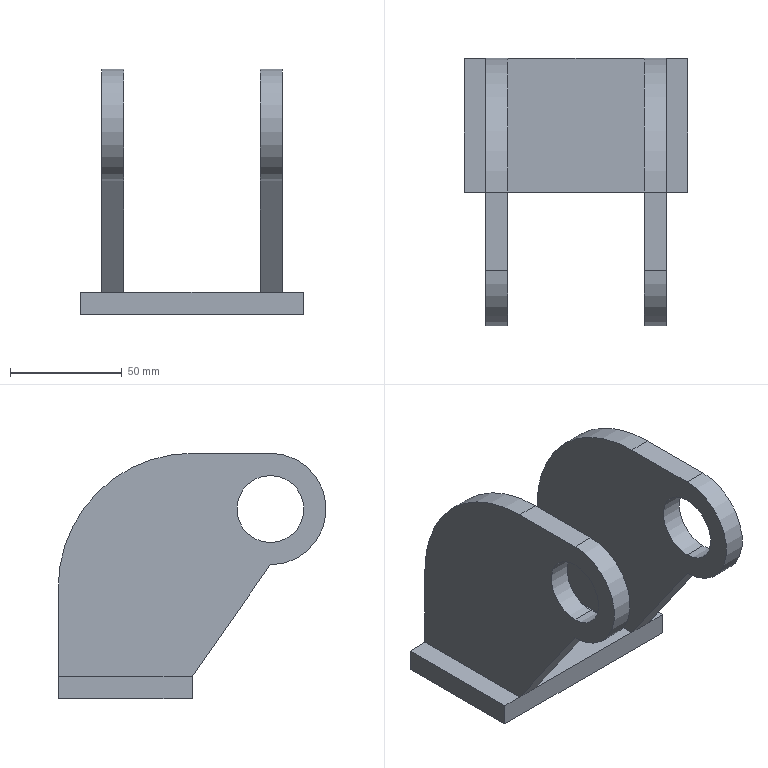Part | STEP file | TN-NHGJQJ-001-002 | 1 solid | 24 faces | box 100 x 120 x 110 mm | volume 222546 mm3 | plane 16 | cylinder 8 | commonest cylinder face diameters 30 x4 50 x2 120 x2
STEP:
#1=CARTESIAN_POINT('',(16.652,-66.545,70.));
#2=VERTEX_POINT('',#1);
#3=CARTESIAN_POINT('',(16.652,-66.545,100.));
#4=VERTEX_POINT('',#3);
#5=CARTESIAN_POINT('',(16.652,-66.545,85.));
#6=DIRECTION('',(-1.,0.,0.));
#7=DIRECTION('',(0.,0.,1.));
#8=AXIS2_PLACEMENT_3D('',#5,#6,#7);
#9=CIRCLE('',#8,15.);
#10=EDGE_CURVE('',#2,#4,#9,.T.);
#11=ORIENTED_EDGE('',*,*,#10,.F.);
#12=CARTESIAN_POINT('',(6.652,-66.545,70.));
#13=VERTEX_POINT('',#12);
#14=CARTESIAN_POINT('',(26.152,-66.545,70.));
#15=DIRECTION('',(-1.,0.,0.));
#16=VECTOR('',#15,1000.);
#17=LINE('',#14,#16);
#18=EDGE_CURVE('',#2,#13,#17,.T.);
#19=ORIENTED_EDGE('',*,*,#18,.T.);
#20=CARTESIAN_POINT('',(6.652,-66.545,100.));
#21=VERTEX_POINT('',#20);
#22=CARTESIAN_POINT('',(6.652,-66.545,85.));
#23=DIRECTION('',(-1.,0.,0.));
#24=DIRECTION('',(0.,0.,1.));
#25=AXIS2_PLACEMENT_3D('',#22,#23,#24);
#26=CIRCLE('',#25,15.);
#27=EDGE_CURVE('',#13,#21,#26,.T.);
#28=ORIENTED_EDGE('',*,*,#27,.T.);
#29=CARTESIAN_POINT('',(26.152,-66.545,100.));
#30=DIRECTION('',(-1.,0.,0.));
#31=VECTOR('',#30,1000.);
#32=LINE('',#29,#31);
#33=EDGE_CURVE('',#4,#21,#32,.T.);
#34=ORIENTED_EDGE('',*,*,#33,.F.);
#35=EDGE_LOOP('',(#11,#19,#28,#34));
#36=FACE_OUTER_BOUND('',#35,.T.);
#37=CARTESIAN_POINT('',(26.152,-66.545,85.));
#38=DIRECTION('',(-1.,0.,0.));
#39=DIRECTION('',(0.,0.,1.));
#40=AXIS2_PLACEMENT_3D('',#37,#38,#39);
#41=CYLINDRICAL_SURFACE('',#40,15.);
#42=ADVANCED_FACE('',(#36),#41,.F.);
#43=CARTESIAN_POINT('',(-54.348,-66.545,100.));
#44=VERTEX_POINT('',#43);
#45=CARTESIAN_POINT('',(-54.348,-66.545,70.));
#46=VERTEX_POINT('',#45);
#47=CARTESIAN_POINT('',(-54.348,-66.545,85.));
#48=DIRECTION('',(1.,0.,0.));
#49=DIRECTION('',(0.,0.,1.));
#50=AXIS2_PLACEMENT_3D('',#47,#48,#49);
#51=CIRCLE('',#50,15.);
#52=EDGE_CURVE('',#44,#46,#51,.T.);
#53=ORIENTED_EDGE('',*,*,#52,.T.);
#54=CARTESIAN_POINT('',(-64.348,-66.545,70.));
#55=VERTEX_POINT('',#54);
#56=CARTESIAN_POINT('',(26.152,-66.545,70.));
#57=DIRECTION('',(-1.,0.,0.));
#58=VECTOR('',#57,1000.);
#59=LINE('',#56,#58);
#60=EDGE_CURVE('',#46,#55,#59,.T.);
#61=ORIENTED_EDGE('',*,*,#60,.T.);
#62=CARTESIAN_POINT('',(-64.348,-66.545,100.));
#63=VERTEX_POINT('',#62);
#64=CARTESIAN_POINT('',(-64.348,-66.545,85.));
#65=DIRECTION('',(-1.,0.,0.));
#66=DIRECTION('',(0.,0.,1.));
#67=AXIS2_PLACEMENT_3D('',#64,#65,#66);
#68=CIRCLE('',#67,15.);
#69=EDGE_CURVE('',#55,#63,#68,.T.);
#70=ORIENTED_EDGE('',*,*,#69,.T.);
#71=CARTESIAN_POINT('',(26.152,-66.545,100.));
#72=DIRECTION('',(-1.,0.,0.));
#73=VECTOR('',#72,1000.);
#74=LINE('',#71,#73);
#75=EDGE_CURVE('',#44,#63,#74,.T.);
#76=ORIENTED_EDGE('',*,*,#75,.F.);
#77=EDGE_LOOP('',(#53,#61,#70,#76));
#78=FACE_OUTER_BOUND('',#77,.T.);
#79=CARTESIAN_POINT('',(26.152,-66.545,85.));
#80=DIRECTION('',(-1.,0.,0.));
#81=DIRECTION('',(0.,0.,1.));
#82=AXIS2_PLACEMENT_3D('',#79,#80,#81);
#83=CYLINDRICAL_SURFACE('',#82,15.);
#84=ADVANCED_FACE('',(#78),#83,.F.);
#85=CARTESIAN_POINT('',(6.652,-66.545,85.));
#86=DIRECTION('',(-1.,0.,0.));
#87=DIRECTION('',(0.,0.,1.));
#88=AXIS2_PLACEMENT_3D('',#85,#86,#87);
#89=CIRCLE('',#88,15.);
#90=EDGE_CURVE('',#21,#13,#89,.T.);
#91=ORIENTED_EDGE('',*,*,#90,.F.);
#92=ORIENTED_EDGE('',*,*,#27,.F.);
#93=EDGE_LOOP('',(#91,#92));
#94=FACE_BOUND('',#93,.T.);
#95=CARTESIAN_POINT('',(6.652,-66.545,60.));
#96=VERTEX_POINT('',#95);
#97=CARTESIAN_POINT('',(6.652,-31.545,10.));
#98=VERTEX_POINT('',#97);
#99=CARTESIAN_POINT('',(6.652,-66.545,60.));
#100=DIRECTION('',(0.,0.5735,-0.8192));
#101=VECTOR('',#100,1000.);
#102=LINE('',#99,#101);
#103=EDGE_CURVE('',#96,#98,#102,.T.);
#104=ORIENTED_EDGE('',*,*,#103,.F.);
#105=CARTESIAN_POINT('',(6.652,-66.545,110.));
#106=VERTEX_POINT('',#105);
#107=CARTESIAN_POINT('',(6.652,-66.545,85.));
#108=DIRECTION('',(1.,0.,0.));
#109=DIRECTION('',(0.,0.,-1.));
#110=AXIS2_PLACEMENT_3D('',#107,#108,#109);
#111=CIRCLE('',#110,25.);
#112=EDGE_CURVE('',#106,#96,#111,.T.);
#113=ORIENTED_EDGE('',*,*,#112,.F.);
#114=CARTESIAN_POINT('',(6.652,-31.545,110.));
#115=VERTEX_POINT('',#114);
#116=CARTESIAN_POINT('',(6.652,28.455,110.));
#117=DIRECTION('',(0.,-1.,0.));
#118=VECTOR('',#117,1000.);
#119=LINE('',#116,#118);
#120=EDGE_CURVE('',#115,#106,#119,.T.);
#121=ORIENTED_EDGE('',*,*,#120,.F.);
#122=CARTESIAN_POINT('',(6.652,28.455,50.));
#123=VERTEX_POINT('',#122);
#124=CARTESIAN_POINT('',(6.652,-31.545,50.));
#125=DIRECTION('',(1.,0.,0.));
#126=DIRECTION('',(0.,0.,-1.));
#127=AXIS2_PLACEMENT_3D('',#124,#125,#126);
#128=CIRCLE('',#127,60.);
#129=EDGE_CURVE('',#123,#115,#128,.T.);
#130=ORIENTED_EDGE('',*,*,#129,.F.);
#131=CARTESIAN_POINT('',(6.652,28.455,10.));
#132=VERTEX_POINT('',#131);
#133=CARTESIAN_POINT('',(6.652,28.455,110.));
#134=DIRECTION('',(0.,0.,1.));
#135=VECTOR('',#134,1000.);
#136=LINE('',#133,#135);
#137=EDGE_CURVE('',#132,#123,#136,.T.);
#138=ORIENTED_EDGE('',*,*,#137,.F.);
#139=CARTESIAN_POINT('',(6.652,28.455,10.));
#140=DIRECTION('',(0.,1.,0.));
#141=VECTOR('',#140,1000.);
#142=LINE('',#139,#141);
#143=EDGE_CURVE('',#98,#132,#142,.T.);
#144=ORIENTED_EDGE('',*,*,#143,.F.);
#145=EDGE_LOOP('',(#104,#113,#121,#130,#138,#144));
#146=FACE_OUTER_BOUND('',#145,.T.);
#147=CARTESIAN_POINT('',(6.652,28.455,110.));
#148=DIRECTION('',(1.,0.,0.));
#149=DIRECTION('',(0.,1.,0.));
#150=AXIS2_PLACEMENT_3D('',#147,#148,#149);
#151=PLANE('',#150);
#152=ADVANCED_FACE('',(#94,#146),#151,.F.);
#153=ORIENTED_EDGE('',*,*,#18,.F.);
#154=CARTESIAN_POINT('',(16.652,-66.545,85.));
#155=DIRECTION('',(-1.,0.,0.));
#156=DIRECTION('',(0.,0.,1.));
#157=AXIS2_PLACEMENT_3D('',#154,#155,#156);
#158=CIRCLE('',#157,15.);
#159=EDGE_CURVE('',#4,#2,#158,.T.);
#160=ORIENTED_EDGE('',*,*,#159,.F.);
#161=ORIENTED_EDGE('',*,*,#33,.T.);
#162=ORIENTED_EDGE('',*,*,#90,.T.);
#163=EDGE_LOOP('',(#153,#160,#161,#162));
#164=FACE_OUTER_BOUND('',#163,.T.);
#165=CARTESIAN_POINT('',(26.152,-66.545,85.));
#166=DIRECTION('',(-1.,0.,0.));
#167=DIRECTION('',(0.,0.,1.));
#168=AXIS2_PLACEMENT_3D('',#165,#166,#167);
#169=CYLINDRICAL_SURFACE('',#168,15.);
#170=ADVANCED_FACE('',(#164),#169,.F.);
#171=CARTESIAN_POINT('',(-54.348,28.455,10.));
#172=VERTEX_POINT('',#171);
#173=CARTESIAN_POINT('',(0.,28.455,10.));
#174=DIRECTION('',(-1.,0.,0.));
#175=VECTOR('',#174,1000.);
#176=LINE('',#173,#175);
#177=EDGE_CURVE('',#132,#172,#176,.T.);
#178=ORIENTED_EDGE('',*,*,#177,.T.);
#179=CARTESIAN_POINT('',(-54.348,-31.545,10.));
#180=VERTEX_POINT('',#179);
#181=CARTESIAN_POINT('',(-54.348,0.,10.));
#182=DIRECTION('',(0.,-1.,0.));
#183=VECTOR('',#182,1000.);
#184=LINE('',#181,#183);
#185=EDGE_CURVE('',#172,#180,#184,.T.);
#186=ORIENTED_EDGE('',*,*,#185,.T.);
#187=CARTESIAN_POINT('',(0.,-31.545,10.));
#188=DIRECTION('',(1.,0.,0.));
#189=VECTOR('',#188,1000.);
#190=LINE('',#187,#189);
#191=EDGE_CURVE('',#180,#98,#190,.T.);
#192=ORIENTED_EDGE('',*,*,#191,.T.);
#193=ORIENTED_EDGE('',*,*,#143,.T.);
#194=EDGE_LOOP('',(#178,#186,#192,#193));
#195=FACE_OUTER_BOUND('',#194,.T.);
#196=CARTESIAN_POINT('',(0.,0.,10.));
#197=DIRECTION('',(0.,0.,1.));
#198=DIRECTION('',(1.,0.,0.));
#199=AXIS2_PLACEMENT_3D('',#196,#197,#198);
#200=PLANE('',#199);
#201=ADVANCED_FACE('',(#195),#200,.T.);
#202=ORIENTED_EDGE('',*,*,#103,.T.);
#203=CARTESIAN_POINT('',(16.652,-31.545,10.));
#204=VERTEX_POINT('',#203);
#205=CARTESIAN_POINT('',(6.652,-31.545,10.));
#206=DIRECTION('',(1.,0.,0.));
#207=VECTOR('',#206,1000.);
#208=LINE('',#205,#207);
#209=EDGE_CURVE('',#98,#204,#208,.T.);
#210=ORIENTED_EDGE('',*,*,#209,.T.);
#211=CARTESIAN_POINT('',(16.652,-66.545,60.));
#212=VERTEX_POINT('',#211);
#213=CARTESIAN_POINT('',(16.652,-31.545,10.));
#214=DIRECTION('',(0.,-0.5735,0.8192));
#215=VECTOR('',#214,1000.);
#216=LINE('',#213,#215);
#217=EDGE_CURVE('',#204,#212,#216,.T.);
#218=ORIENTED_EDGE('',*,*,#217,.T.);
#219=CARTESIAN_POINT('',(6.652,-66.545,60.));
#220=DIRECTION('',(-1.,0.,0.));
#221=VECTOR('',#220,1000.);
#222=LINE('',#219,#221);
#223=EDGE_CURVE('',#212,#96,#222,.T.);
#224=ORIENTED_EDGE('',*,*,#223,.T.);
#225=EDGE_LOOP('',(#202,#210,#218,#224));
#226=FACE_OUTER_BOUND('',#225,.T.);
#227=CARTESIAN_POINT('',(6.652,-31.545,10.));
#228=DIRECTION('',(0.,-0.8192,-0.5735));
#229=DIRECTION('',(0.,0.5735,-0.8192));
#230=AXIS2_PLACEMENT_3D('',#227,#228,#229);
#231=PLANE('',#230);
#232=ADVANCED_FACE('',(#226),#231,.T.);
#233=CARTESIAN_POINT('',(16.652,-66.545,110.));
#234=VERTEX_POINT('',#233);
#235=CARTESIAN_POINT('',(16.652,-66.545,85.));
#236=DIRECTION('',(-1.,0.,0.));
#237=DIRECTION('',(0.,0.,-1.));
#238=AXIS2_PLACEMENT_3D('',#235,#236,#237);
#239=CIRCLE('',#238,25.);
#240=EDGE_CURVE('',#212,#234,#239,.T.);
#241=ORIENTED_EDGE('',*,*,#240,.T.);
#242=CARTESIAN_POINT('',(0.,-66.545,110.));
#243=DIRECTION('',(-1.,0.,0.));
#244=VECTOR('',#243,1000.);
#245=LINE('',#242,#244);
#246=EDGE_CURVE('',#234,#106,#245,.T.);
#247=ORIENTED_EDGE('',*,*,#246,.T.);
#248=ORIENTED_EDGE('',*,*,#112,.T.);
#249=ORIENTED_EDGE('',*,*,#223,.F.);
#250=EDGE_LOOP('',(#241,#247,#248,#249));
#251=FACE_OUTER_BOUND('',#250,.T.);
#252=CARTESIAN_POINT('',(0.,-66.545,85.));
#253=DIRECTION('',(1.,0.,0.));
#254=DIRECTION('',(0.,0.,-1.));
#255=AXIS2_PLACEMENT_3D('',#252,#253,#254);
#256=CYLINDRICAL_SURFACE('',#255,25.);
#257=ADVANCED_FACE('',(#251),#256,.T.);
#258=CARTESIAN_POINT('',(16.652,-31.545,110.));
#259=VERTEX_POINT('',#258);
#260=CARTESIAN_POINT('',(16.652,0.,110.));
#261=DIRECTION('',(0.,1.,0.));
#262=VECTOR('',#261,1000.);
#263=LINE('',#260,#262);
#264=EDGE_CURVE('',#234,#259,#263,.T.);
#265=ORIENTED_EDGE('',*,*,#264,.T.);
#266=CARTESIAN_POINT('',(0.,-31.545,110.));
#267=DIRECTION('',(-1.,0.,0.));
#268=VECTOR('',#267,1000.);
#269=LINE('',#266,#268);
#270=EDGE_CURVE('',#259,#115,#269,.T.);
#271=ORIENTED_EDGE('',*,*,#270,.T.);
#272=ORIENTED_EDGE('',*,*,#120,.T.);
#273=ORIENTED_EDGE('',*,*,#246,.F.);
#274=EDGE_LOOP('',(#265,#271,#272,#273));
#275=FACE_OUTER_BOUND('',#274,.T.);
#276=CARTESIAN_POINT('',(0.,0.,110.));
#277=DIRECTION('',(0.,0.,1.));
#278=DIRECTION('',(1.,0.,0.));
#279=AXIS2_PLACEMENT_3D('',#276,#277,#278);
#280=PLANE('',#279);
#281=ADVANCED_FACE('',(#275),#280,.T.);
#282=ORIENTED_EDGE('',*,*,#129,.T.);
#283=ORIENTED_EDGE('',*,*,#270,.F.);
#284=CARTESIAN_POINT('',(16.652,28.455,50.));
#285=VERTEX_POINT('',#284);
#286=CARTESIAN_POINT('',(16.652,-31.545,50.));
#287=DIRECTION('',(-1.,0.,0.));
#288=DIRECTION('',(0.,0.,-1.));
#289=AXIS2_PLACEMENT_3D('',#286,#287,#288);
#290=CIRCLE('',#289,60.);
#291=EDGE_CURVE('',#259,#285,#290,.T.);
#292=ORIENTED_EDGE('',*,*,#291,.T.);
#293=CARTESIAN_POINT('',(0.,28.455,50.));
#294=DIRECTION('',(-1.,0.,0.));
#295=VECTOR('',#294,1000.);
#296=LINE('',#293,#295);
#297=EDGE_CURVE('',#285,#123,#296,.T.);
#298=ORIENTED_EDGE('',*,*,#297,.T.);
#299=EDGE_LOOP('',(#282,#283,#292,#298));
#300=FACE_OUTER_BOUND('',#299,.T.);
#301=CARTESIAN_POINT('',(0.,-31.545,50.));
#302=DIRECTION('',(1.,0.,0.));
#303=DIRECTION('',(0.,0.,-1.));
#304=AXIS2_PLACEMENT_3D('',#301,#302,#303);
#305=CYLINDRICAL_SURFACE('',#304,60.);
#306=ADVANCED_FACE('',(#300),#305,.T.);
#307=ORIENTED_EDGE('',*,*,#297,.F.);
#308=CARTESIAN_POINT('',(16.652,28.455,10.));
#309=VERTEX_POINT('',#308);
#310=CARTESIAN_POINT('',(16.652,28.455,10.));
#311=DIRECTION('',(0.,0.,1.));
#312=VECTOR('',#311,1000.);
#313=LINE('',#310,#312);
#314=EDGE_CURVE('',#309,#285,#313,.T.);
#315=ORIENTED_EDGE('',*,*,#314,.F.);
#316=CARTESIAN_POINT('',(26.152,28.455,10.));
#317=VERTEX_POINT('',#316);
#318=CARTESIAN_POINT('',(-73.848,28.455,10.));
#319=DIRECTION('',(-1.,0.,0.));
#320=VECTOR('',#319,1000.);
#321=LINE('',#318,#320);
#322=EDGE_CURVE('',#317,#309,#321,.T.);
#323=ORIENTED_EDGE('',*,*,#322,.F.);
#324=CARTESIAN_POINT('',(26.152,28.455,0.));
#325=VERTEX_POINT('',#324);
#326=CARTESIAN_POINT('',(26.152,28.455,10.));
#327=DIRECTION('',(0.,0.,1.));
#328=VECTOR('',#327,1000.);
#329=LINE('',#326,#328);
#330=EDGE_CURVE('',#325,#317,#329,.T.);
#331=ORIENTED_EDGE('',*,*,#330,.F.);
#332=CARTESIAN_POINT('',(-73.848,28.455,0.));
#333=VERTEX_POINT('',#332);
#334=CARTESIAN_POINT('',(-73.848,28.455,0.));
#335=DIRECTION('',(1.,0.,0.));
#336=VECTOR('',#335,1000.);
#337=LINE('',#334,#336);
#338=EDGE_CURVE('',#333,#325,#337,.T.);
#339=ORIENTED_EDGE('',*,*,#338,.F.);
#340=CARTESIAN_POINT('',(-73.848,28.455,10.));
#341=VERTEX_POINT('',#340);
#342=CARTESIAN_POINT('',(-73.848,28.455,10.));
#343=DIRECTION('',(0.,0.,-1.));
#344=VECTOR('',#343,1000.);
#345=LINE('',#342,#344);
#346=EDGE_CURVE('',#341,#333,#345,.T.);
#347=ORIENTED_EDGE('',*,*,#346,.F.);
#348=CARTESIAN_POINT('',(-64.348,28.455,10.));
#349=VERTEX_POINT('',#348);
#350=CARTESIAN_POINT('',(-73.848,28.455,10.));
#351=DIRECTION('',(-1.,0.,0.));
#352=VECTOR('',#351,1000.);
#353=LINE('',#350,#352);
#354=EDGE_CURVE('',#349,#341,#353,.T.);
#355=ORIENTED_EDGE('',*,*,#354,.F.);
#356=CARTESIAN_POINT('',(-64.348,28.455,50.));
#357=VERTEX_POINT('',#356);
#358=CARTESIAN_POINT('',(-64.348,28.455,10.));
#359=DIRECTION('',(0.,0.,-1.));
#360=VECTOR('',#359,1000.);
#361=LINE('',#358,#360);
#362=EDGE_CURVE('',#357,#349,#361,.T.);
#363=ORIENTED_EDGE('',*,*,#362,.F.);
#364=CARTESIAN_POINT('',(-54.348,28.455,50.));
#365=VERTEX_POINT('',#364);
#366=CARTESIAN_POINT('',(-73.848,28.455,50.));
#367=DIRECTION('',(-1.,0.,0.));
#368=VECTOR('',#367,1000.);
#369=LINE('',#366,#368);
#370=EDGE_CURVE('',#365,#357,#369,.T.);
#371=ORIENTED_EDGE('',*,*,#370,.F.);
#372=CARTESIAN_POINT('',(-54.348,28.455,10.));
#373=DIRECTION('',(0.,0.,1.));
#374=VECTOR('',#373,1000.);
#375=LINE('',#372,#374);
#376=EDGE_CURVE('',#172,#365,#375,.T.);
#377=ORIENTED_EDGE('',*,*,#376,.F.);
#378=ORIENTED_EDGE('',*,*,#177,.F.);
#379=ORIENTED_EDGE('',*,*,#137,.T.);
#380=EDGE_LOOP('',(#307,#315,#323,#331,#339,#347,#355,#363,#371,#377,#378,#379));
#381=FACE_OUTER_BOUND('',#380,.T.);
#382=CARTESIAN_POINT('',(-73.848,28.455,10.));
#383=DIRECTION('',(0.,-1.,0.));
#384=DIRECTION('',(0.,0.,-1.));
#385=AXIS2_PLACEMENT_3D('',#382,#383,#384);
#386=PLANE('',#385);
#387=ADVANCED_FACE('',(#381),#386,.F.);
#388=ORIENTED_EDGE('',*,*,#159,.T.);
#389=ORIENTED_EDGE('',*,*,#10,.T.);
#390=EDGE_LOOP('',(#388,#389));
#391=FACE_BOUND('',#390,.T.);
#392=CARTESIAN_POINT('',(16.652,28.455,10.));
#393=DIRECTION('',(0.,-1.,0.));
#394=VECTOR('',#393,1000.);
#395=LINE('',#392,#394);
#396=EDGE_CURVE('',#309,#204,#395,.T.);
#397=ORIENTED_EDGE('',*,*,#396,.F.);
#398=ORIENTED_EDGE('',*,*,#314,.T.);
#399=ORIENTED_EDGE('',*,*,#291,.F.);
#400=ORIENTED_EDGE('',*,*,#264,.F.);
#401=ORIENTED_EDGE('',*,*,#240,.F.);
#402=ORIENTED_EDGE('',*,*,#217,.F.);
#403=EDGE_LOOP('',(#397,#398,#399,#400,#401,#402));
#404=FACE_OUTER_BOUND('',#403,.T.);
#405=CARTESIAN_POINT('',(16.652,28.455,110.));
#406=DIRECTION('',(-1.,0.,0.));
#407=DIRECTION('',(0.,-1.,0.));
#408=AXIS2_PLACEMENT_3D('',#405,#406,#407);
#409=PLANE('',#408);
#410=ADVANCED_FACE('',(#391,#404),#409,.F.);
#411=ORIENTED_EDGE('',*,*,#52,.F.);
#412=CARTESIAN_POINT('',(-54.348,-66.545,85.));
#413=DIRECTION('',(1.,0.,0.));
#414=DIRECTION('',(0.,0.,1.));
#415=AXIS2_PLACEMENT_3D('',#412,#413,#414);
#416=CIRCLE('',#415,15.);
#417=EDGE_CURVE('',#46,#44,#416,.T.);
#418=ORIENTED_EDGE('',*,*,#417,.F.);
#419=EDGE_LOOP('',(#411,#418));
#420=FACE_BOUND('',#419,.T.);
#421=ORIENTED_EDGE('',*,*,#185,.F.);
#422=ORIENTED_EDGE('',*,*,#376,.T.);
#423=CARTESIAN_POINT('',(-54.348,-31.545,110.));
#424=VERTEX_POINT('',#423);
#425=CARTESIAN_POINT('',(-54.348,-31.545,50.));
#426=DIRECTION('',(-1.,0.,0.));
#427=DIRECTION('',(0.,0.,-1.));
#428=AXIS2_PLACEMENT_3D('',#425,#426,#427);
#429=CIRCLE('',#428,60.);
#430=EDGE_CURVE('',#424,#365,#429,.T.);
#431=ORIENTED_EDGE('',*,*,#430,.F.);
#432=CARTESIAN_POINT('',(-54.348,-66.545,110.));
#433=VERTEX_POINT('',#432);
#434=CARTESIAN_POINT('',(-54.348,28.455,110.));
#435=DIRECTION('',(0.,1.,0.));
#436=VECTOR('',#435,1000.);
#437=LINE('',#434,#436);
#438=EDGE_CURVE('',#433,#424,#437,.T.);
#439=ORIENTED_EDGE('',*,*,#438,.F.);
#440=CARTESIAN_POINT('',(-54.348,-66.545,60.));
#441=VERTEX_POINT('',#440);
#442=CARTESIAN_POINT('',(-54.348,-66.545,85.));
#443=DIRECTION('',(-1.,0.,0.));
#444=DIRECTION('',(0.,0.,1.));
#445=AXIS2_PLACEMENT_3D('',#442,#443,#444);
#446=CIRCLE('',#445,25.);
#447=EDGE_CURVE('',#441,#433,#446,.T.);
#448=ORIENTED_EDGE('',*,*,#447,.F.);
#449=CARTESIAN_POINT('',(-54.348,-31.545,10.));
#450=DIRECTION('',(0.,-0.5735,0.8192));
#451=VECTOR('',#450,1000.);
#452=LINE('',#449,#451);
#453=EDGE_CURVE('',#180,#441,#452,.T.);
#454=ORIENTED_EDGE('',*,*,#453,.F.);
#455=EDGE_LOOP('',(#421,#422,#431,#439,#448,#454));
#456=FACE_OUTER_BOUND('',#455,.T.);
#457=CARTESIAN_POINT('',(-54.348,28.455,110.));
#458=DIRECTION('',(-1.,0.,0.));
#459=DIRECTION('',(0.,-1.,0.));
#460=AXIS2_PLACEMENT_3D('',#457,#458,#459);
#461=PLANE('',#460);
#462=ADVANCED_FACE('',(#420,#456),#461,.F.);
#463=ORIENTED_EDGE('',*,*,#209,.F.);
#464=ORIENTED_EDGE('',*,*,#191,.F.);
#465=CARTESIAN_POINT('',(-64.348,-31.545,10.));
#466=VERTEX_POINT('',#465);
#467=CARTESIAN_POINT('',(-73.848,-31.545,10.));
#468=DIRECTION('',(1.,0.,0.));
#469=VECTOR('',#468,1000.);
#470=LINE('',#467,#469);
#471=EDGE_CURVE('',#466,#180,#470,.T.);
#472=ORIENTED_EDGE('',*,*,#471,.F.);
#473=CARTESIAN_POINT('',(-73.848,-31.545,10.));
#474=VERTEX_POINT('',#473);
#475=CARTESIAN_POINT('',(-73.848,-31.545,10.));
#476=DIRECTION('',(1.,0.,0.));
#477=VECTOR('',#476,1000.);
#478=LINE('',#475,#477);
#479=EDGE_CURVE('',#474,#466,#478,.T.);
#480=ORIENTED_EDGE('',*,*,#479,.F.);
#481=CARTESIAN_POINT('',(-73.848,-31.545,0.));
#482=VERTEX_POINT('',#481);
#483=CARTESIAN_POINT('',(-73.848,-31.545,10.));
#484=DIRECTION('',(0.,0.,1.));
#485=VECTOR('',#484,1000.);
#486=LINE('',#483,#485);
#487=EDGE_CURVE('',#482,#474,#486,.T.);
#488=ORIENTED_EDGE('',*,*,#487,.F.);
#489=CARTESIAN_POINT('',(26.152,-31.545,0.));
#490=VERTEX_POINT('',#489);
#491=CARTESIAN_POINT('',(-73.848,-31.545,0.));
#492=DIRECTION('',(-1.,0.,0.));
#493=VECTOR('',#492,1000.);
#494=LINE('',#491,#493);
#495=EDGE_CURVE('',#490,#482,#494,.T.);
#496=ORIENTED_EDGE('',*,*,#495,.F.);
#497=CARTESIAN_POINT('',(26.152,-31.545,10.));
#498=VERTEX_POINT('',#497);
#499=CARTESIAN_POINT('',(26.152,-31.545,10.));
#500=DIRECTION('',(0.,0.,-1.));
#501=VECTOR('',#500,1000.);
#502=LINE('',#499,#501);
#503=EDGE_CURVE('',#498,#490,#502,.T.);
#504=ORIENTED_EDGE('',*,*,#503,.F.);
#505=CARTESIAN_POINT('',(-73.848,-31.545,10.));
#506=DIRECTION('',(1.,0.,0.));
#507=VECTOR('',#506,1000.);
#508=LINE('',#505,#507);
#509=EDGE_CURVE('',#204,#498,#508,.T.);
#510=ORIENTED_EDGE('',*,*,#509,.F.);
#511=EDGE_LOOP('',(#463,#464,#472,#480,#488,#496,#504,#510));
#512=FACE_OUTER_BOUND('',#511,.T.);
#513=CARTESIAN_POINT('',(-73.848,-31.545,10.));
#514=DIRECTION('',(0.,1.,0.));
#515=DIRECTION('',(0.,0.,1.));
#516=AXIS2_PLACEMENT_3D('',#513,#514,#515);
#517=PLANE('',#516);
#518=ADVANCED_FACE('',(#512),#517,.F.);
#519=ORIENTED_EDGE('',*,*,#509,.T.);
#520=CARTESIAN_POINT('',(26.152,0.,10.));
#521=DIRECTION('',(0.,1.,0.));
#522=VECTOR('',#521,1000.);
#523=LINE('',#520,#522);
#524=EDGE_CURVE('',#498,#317,#523,.T.);
#525=ORIENTED_EDGE('',*,*,#524,.T.);
#526=ORIENTED_EDGE('',*,*,#322,.T.);
#527=ORIENTED_EDGE('',*,*,#396,.T.);
#528=EDGE_LOOP('',(#519,#525,#526,#527));
#529=FACE_OUTER_BOUND('',#528,.T.);
#530=CARTESIAN_POINT('',(0.,0.,10.));
#531=DIRECTION('',(0.,0.,1.));
#532=DIRECTION('',(1.,0.,0.));
#533=AXIS2_PLACEMENT_3D('',#530,#531,#532);
#534=PLANE('',#533);
#535=ADVANCED_FACE('',(#529),#534,.T.);
#536=ORIENTED_EDGE('',*,*,#330,.T.);
#537=ORIENTED_EDGE('',*,*,#524,.F.);
#538=ORIENTED_EDGE('',*,*,#503,.T.);
#539=CARTESIAN_POINT('',(26.152,28.455,0.));
#540=DIRECTION('',(0.,-1.,0.));
#541=VECTOR('',#540,1000.);
#542=LINE('',#539,#541);
#543=EDGE_CURVE('',#325,#490,#542,.T.);
#544=ORIENTED_EDGE('',*,*,#543,.F.);
#545=EDGE_LOOP('',(#536,#537,#538,#544));
#546=FACE_OUTER_BOUND('',#545,.T.);
#547=CARTESIAN_POINT('',(26.152,28.455,10.));
#548=DIRECTION('',(-1.,0.,0.));
#549=DIRECTION('',(0.,-1.,0.));
#550=AXIS2_PLACEMENT_3D('',#547,#548,#549);
#551=PLANE('',#550);
#552=ADVANCED_FACE('',(#546),#551,.F.);
#553=ORIENTED_EDGE('',*,*,#338,.T.);
#554=ORIENTED_EDGE('',*,*,#543,.T.);
#555=ORIENTED_EDGE('',*,*,#495,.T.);
#556=CARTESIAN_POINT('',(-73.848,0.,0.));
#557=DIRECTION('',(0.,-1.,0.));
#558=VECTOR('',#557,1000.);
#559=LINE('',#556,#558);
#560=EDGE_CURVE('',#333,#482,#559,.T.);
#561=ORIENTED_EDGE('',*,*,#560,.F.);
#562=EDGE_LOOP('',(#553,#554,#555,#561));
#563=FACE_OUTER_BOUND('',#562,.T.);
#564=CARTESIAN_POINT('',(0.,0.,0.));
#565=DIRECTION('',(0.,0.,1.));
#566=DIRECTION('',(1.,0.,0.));
#567=AXIS2_PLACEMENT_3D('',#564,#565,#566);
#568=PLANE('',#567);
#569=ADVANCED_FACE('',(#563),#568,.F.);
#570=ORIENTED_EDGE('',*,*,#487,.T.);
#571=CARTESIAN_POINT('',(-73.848,28.455,10.));
#572=DIRECTION('',(0.,-1.,0.));
#573=VECTOR('',#572,1000.);
#574=LINE('',#571,#573);
#575=EDGE_CURVE('',#341,#474,#574,.T.);
#576=ORIENTED_EDGE('',*,*,#575,.F.);
#577=ORIENTED_EDGE('',*,*,#346,.T.);
#578=ORIENTED_EDGE('',*,*,#560,.T.);
#579=EDGE_LOOP('',(#570,#576,#577,#578));
#580=FACE_OUTER_BOUND('',#579,.T.);
#581=CARTESIAN_POINT('',(-73.848,28.455,10.));
#582=DIRECTION('',(1.,0.,0.));
#583=DIRECTION('',(0.,0.,-1.));
#584=AXIS2_PLACEMENT_3D('',#581,#582,#583);
#585=PLANE('',#584);
#586=ADVANCED_FACE('',(#580),#585,.F.);
#587=ORIENTED_EDGE('',*,*,#575,.T.);
#588=ORIENTED_EDGE('',*,*,#479,.T.);
#589=CARTESIAN_POINT('',(-64.348,0.,10.));
#590=DIRECTION('',(0.,1.,0.));
#591=VECTOR('',#590,1000.);
#592=LINE('',#589,#591);
#593=EDGE_CURVE('',#466,#349,#592,.T.);
#594=ORIENTED_EDGE('',*,*,#593,.T.);
#595=ORIENTED_EDGE('',*,*,#354,.T.);
#596=EDGE_LOOP('',(#587,#588,#594,#595));
#597=FACE_OUTER_BOUND('',#596,.T.);
#598=CARTESIAN_POINT('',(0.,0.,10.));
#599=DIRECTION('',(0.,0.,1.));
#600=DIRECTION('',(1.,0.,0.));
#601=AXIS2_PLACEMENT_3D('',#598,#599,#600);
#602=PLANE('',#601);
#603=ADVANCED_FACE('',(#597),#602,.T.);
#604=CARTESIAN_POINT('',(-64.348,-66.545,85.));
#605=DIRECTION('',(-1.,0.,0.));
#606=DIRECTION('',(0.,0.,1.));
#607=AXIS2_PLACEMENT_3D('',#604,#605,#606);
#608=CIRCLE('',#607,15.);
#609=EDGE_CURVE('',#63,#55,#608,.T.);
#610=ORIENTED_EDGE('',*,*,#609,.F.);
#611=ORIENTED_EDGE('',*,*,#69,.F.);
#612=EDGE_LOOP('',(#610,#611));
#613=FACE_BOUND('',#612,.T.);
#614=CARTESIAN_POINT('',(-64.348,-66.545,60.));
#615=VERTEX_POINT('',#614);
#616=CARTESIAN_POINT('',(-64.348,-66.545,60.));
#617=DIRECTION('',(0.,0.5735,-0.8192));
#618=VECTOR('',#617,1000.);
#619=LINE('',#616,#618);
#620=EDGE_CURVE('',#615,#466,#619,.T.);
#621=ORIENTED_EDGE('',*,*,#620,.F.);
#622=CARTESIAN_POINT('',(-64.348,-66.545,110.));
#623=VERTEX_POINT('',#622);
#624=CARTESIAN_POINT('',(-64.348,-66.545,85.));
#625=DIRECTION('',(1.,0.,0.));
#626=DIRECTION('',(0.,0.,1.));
#627=AXIS2_PLACEMENT_3D('',#624,#625,#626);
#628=CIRCLE('',#627,25.);
#629=EDGE_CURVE('',#623,#615,#628,.T.);
#630=ORIENTED_EDGE('',*,*,#629,.F.);
#631=CARTESIAN_POINT('',(-64.348,-31.545,110.));
#632=VERTEX_POINT('',#631);
#633=CARTESIAN_POINT('',(-64.348,28.455,110.));
#634=DIRECTION('',(0.,-1.,0.));
#635=VECTOR('',#634,1000.);
#636=LINE('',#633,#635);
#637=EDGE_CURVE('',#632,#623,#636,.T.);
#638=ORIENTED_EDGE('',*,*,#637,.F.);
#639=CARTESIAN_POINT('',(-64.348,-31.545,50.));
#640=DIRECTION('',(1.,0.,0.));
#641=DIRECTION('',(0.,0.,-1.));
#642=AXIS2_PLACEMENT_3D('',#639,#640,#641);
#643=CIRCLE('',#642,60.);
#644=EDGE_CURVE('',#357,#632,#643,.T.);
#645=ORIENTED_EDGE('',*,*,#644,.F.);
#646=ORIENTED_EDGE('',*,*,#362,.T.);
#647=ORIENTED_EDGE('',*,*,#593,.F.);
#648=EDGE_LOOP('',(#621,#630,#638,#645,#646,#647));
#649=FACE_OUTER_BOUND('',#648,.T.);
#650=CARTESIAN_POINT('',(-64.348,28.455,110.));
#651=DIRECTION('',(1.,0.,0.));
#652=DIRECTION('',(0.,0.,-1.));
#653=AXIS2_PLACEMENT_3D('',#650,#651,#652);
#654=PLANE('',#653);
#655=ADVANCED_FACE('',(#613,#649),#654,.F.);
#656=ORIENTED_EDGE('',*,*,#644,.T.);
#657=CARTESIAN_POINT('',(0.,-31.545,110.));
#658=DIRECTION('',(1.,0.,0.));
#659=VECTOR('',#658,1000.);
#660=LINE('',#657,#659);
#661=EDGE_CURVE('',#632,#424,#660,.T.);
#662=ORIENTED_EDGE('',*,*,#661,.T.);
#663=ORIENTED_EDGE('',*,*,#430,.T.);
#664=ORIENTED_EDGE('',*,*,#370,.T.);
#665=EDGE_LOOP('',(#656,#662,#663,#664));
#666=FACE_OUTER_BOUND('',#665,.T.);
#667=CARTESIAN_POINT('',(0.,-31.545,50.));
#668=DIRECTION('',(1.,0.,0.));
#669=DIRECTION('',(0.,0.,-1.));
#670=AXIS2_PLACEMENT_3D('',#667,#668,#669);
#671=CYLINDRICAL_SURFACE('',#670,60.);
#672=ADVANCED_FACE('',(#666),#671,.T.);
#673=ORIENTED_EDGE('',*,*,#60,.F.);
#674=ORIENTED_EDGE('',*,*,#417,.T.);
#675=ORIENTED_EDGE('',*,*,#75,.T.);
#676=ORIENTED_EDGE('',*,*,#609,.T.);
#677=EDGE_LOOP('',(#673,#674,#675,#676));
#678=FACE_OUTER_BOUND('',#677,.T.);
#679=CARTESIAN_POINT('',(26.152,-66.545,85.));
#680=DIRECTION('',(-1.,0.,0.));
#681=DIRECTION('',(0.,0.,1.));
#682=AXIS2_PLACEMENT_3D('',#679,#680,#681);
#683=CYLINDRICAL_SURFACE('',#682,15.);
#684=ADVANCED_FACE('',(#678),#683,.F.);
#685=ORIENTED_EDGE('',*,*,#453,.T.);
#686=CARTESIAN_POINT('',(-54.348,-66.545,60.));
#687=DIRECTION('',(-1.,0.,0.));
#688=VECTOR('',#687,1000.);
#689=LINE('',#686,#688);
#690=EDGE_CURVE('',#441,#615,#689,.T.);
#691=ORIENTED_EDGE('',*,*,#690,.T.);
#692=ORIENTED_EDGE('',*,*,#620,.T.);
#693=ORIENTED_EDGE('',*,*,#471,.T.);
#694=EDGE_LOOP('',(#685,#691,#692,#693));
#695=FACE_OUTER_BOUND('',#694,.T.);
#696=CARTESIAN_POINT('',(-54.348,-31.545,10.));
#697=DIRECTION('',(0.,-0.8192,-0.5735));
#698=DIRECTION('',(0.,0.5735,-0.8192));
#699=AXIS2_PLACEMENT_3D('',#696,#697,#698);
#700=PLANE('',#699);
#701=ADVANCED_FACE('',(#695),#700,.T.);
#702=ORIENTED_EDGE('',*,*,#438,.T.);
#703=ORIENTED_EDGE('',*,*,#661,.F.);
#704=ORIENTED_EDGE('',*,*,#637,.T.);
#705=CARTESIAN_POINT('',(0.,-66.545,110.));
#706=DIRECTION('',(1.,0.,0.));
#707=VECTOR('',#706,1000.);
#708=LINE('',#705,#707);
#709=EDGE_CURVE('',#623,#433,#708,.T.);
#710=ORIENTED_EDGE('',*,*,#709,.T.);
#711=EDGE_LOOP('',(#702,#703,#704,#710));
#712=FACE_OUTER_BOUND('',#711,.T.);
#713=CARTESIAN_POINT('',(0.,0.,110.));
#714=DIRECTION('',(0.,0.,1.));
#715=DIRECTION('',(1.,0.,0.));
#716=AXIS2_PLACEMENT_3D('',#713,#714,#715);
#717=PLANE('',#716);
#718=ADVANCED_FACE('',(#712),#717,.T.);
#719=ORIENTED_EDGE('',*,*,#709,.F.);
#720=ORIENTED_EDGE('',*,*,#629,.T.);
#721=ORIENTED_EDGE('',*,*,#690,.F.);
#722=ORIENTED_EDGE('',*,*,#447,.T.);
#723=EDGE_LOOP('',(#719,#720,#721,#722));
#724=FACE_OUTER_BOUND('',#723,.T.);
#725=CARTESIAN_POINT('',(0.,-66.545,85.));
#726=DIRECTION('',(-1.,0.,0.));
#727=DIRECTION('',(0.,0.,1.));
#728=AXIS2_PLACEMENT_3D('',#725,#726,#727);
#729=CYLINDRICAL_SURFACE('',#728,25.);
#730=ADVANCED_FACE('',(#724),#729,.T.);
#731=CLOSED_SHELL('',(#42,#84,#152,#170,#201,#232,#257,#281,#306,#387,#410,#462,#518,#535,#552,#569,#586,#603,#655,#672,#684,#701,#718,#730));
#732=MANIFOLD_SOLID_BREP('',#731);
#733=CARTESIAN_POINT('',(0.,0.,0.));
#734=DIRECTION('',(0.,0.,1.));
#735=DIRECTION('',(1.,0.,0.));
#736=AXIS2_PLACEMENT_3D('',#733,#734,#735);
#737=(LENGTH_UNIT()NAMED_UNIT(*)SI_UNIT(.MILLI.,.METRE.));
#738=UNCERTAINTY_MEASURE_WITH_UNIT(LENGTH_MEASURE(0.00001),#737,'','');
#739=(NAMED_UNIT(*)PLANE_ANGLE_UNIT()SI_UNIT($,.RADIAN.));
#740=(NAMED_UNIT(*)SI_UNIT($,.STERADIAN.)SOLID_ANGLE_UNIT());
#741=(GEOMETRIC_REPRESENTATION_CONTEXT(3)GLOBAL_UNCERTAINTY_ASSIGNED_CONTEXT((#738))GLOBAL_UNIT_ASSIGNED_CONTEXT((#737,#739,#740))REPRESENTATION_CONTEXT('',''));
#742=ADVANCED_BREP_SHAPE_REPRESENTATION('',(#732,#736),#741);